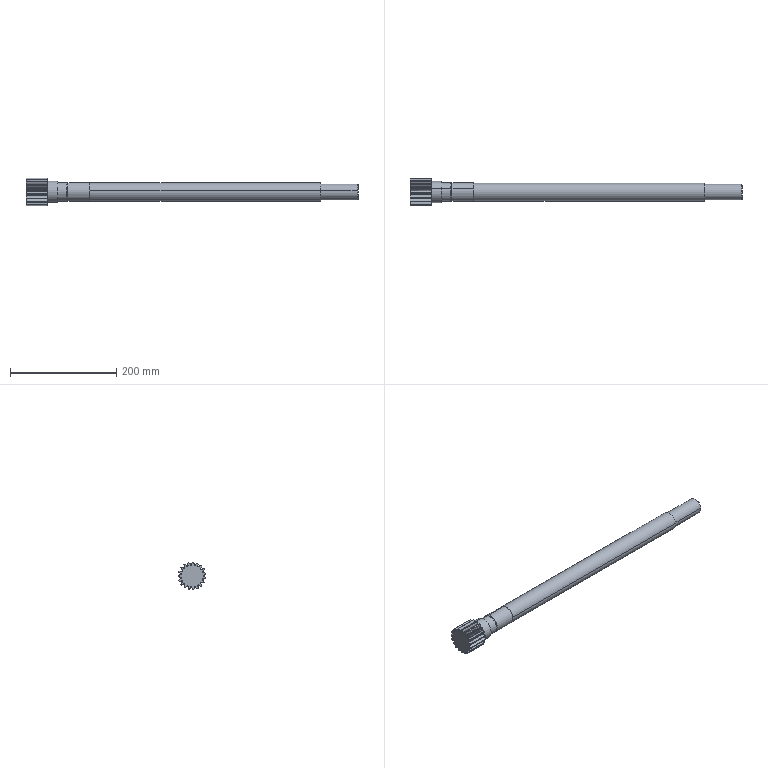Part | NX | features BREP 1 | 1 solid | 118 faces | box 624.795 x 52.296 x 52.433 mm | volume 595829 mm3 | cylinder 50 | spline 38 | plane 26 | cone 2 | torus 2 | commonest cylinder face diameters 41.25 x19 52.5 x19 35 x4 30 x2 32 x2 33.982 x2